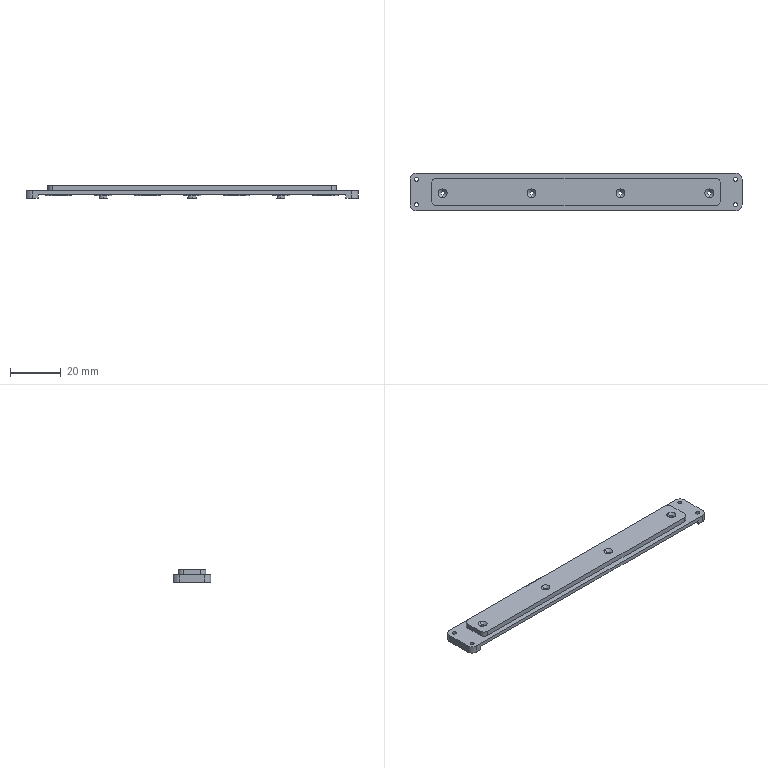NC program | NX | posted with a generic post | part box 130.666 x 14.95 x 5 mm
Lines 1701 to 3662 of 3855, first 1713 of 1960 lines:
(CAVITY_MILL_COPY_COPY , TOOL : D2)
N3370 T02 M6
N3372 G54
N3374 G17 G0 G90 X50.631 Y-0.725 S9500 M3
N3376 G43 Z30. H2
N3378 Z-0.125
N3380 G94 G1 Z-1.125 F1000.
N3382 X50.588 Y-0.761
N3384 G3 X50.231 Y-1.527 R1.
N3386 G1 Y-2.675 F1100.
N3388 X51.379
N3390 G3 X52.145 Y-2.318 R1.
N3392 G1 X52.181 Y-2.275
N3394 Z-0.125
N3396 G0 X50.631 Y-0.725 Z-0.25
N3398 G1 Z-1.25 F1000.
N3400 X50.588 Y-0.761
N3402 G3 X50.231 Y-1.527 R1.
N3404 G1 Y-2.675 F1100.
N3406 X51.379
N3408 G3 X52.145 Y-2.318 R1.
N3410 G1 X52.181 Y-2.275
N3412 Z-0.25
N3414 G0 X50.631 Y-0.725 Z-0.375
N3416 G1 Z-1.375 F1000.
N3418 X50.588 Y-0.761
N3420 G3 X50.231 Y-1.527 R1.
N3422 G1 Y-2.675 F1100.
N3424 X51.379
N3426 G3 X52.145 Y-2.318 R1.
N3428 G1 X52.181 Y-2.275
N3430 Z-0.375
N3432 G0 X50.631 Y-0.725 Z-0.5
N3434 G1 Z-1.5 F1000.
N3436 X50.588 Y-0.761
N3438 G3 X50.231 Y-1.527 R1.
N3440 G1 Y-2.675 F1100.
N3442 X51.379
N3444 G3 X52.145 Y-2.318 R1.
N3446 G1 X52.181 Y-2.275
N3448 Z-0.5
N3450 G0 X50.631 Y-0.725 Z-0.65
N3452 G1 Z-1.65 F1000.
N3454 X50.588 Y-0.761
N3456 G3 X50.231 Y-1.527 R1.
N3458 G1 Y-2.675 F1100.
N3460 X51.379
N3462 G3 X52.145 Y-2.318 R1.
N3464 G1 X52.181 Y-2.275
N3466 Z-0.65
N3468 G0 X50.631 Y-0.725 Z-0.8
N3470 G1 Z-1.8 F1000.
N3472 X50.588 Y-0.761
N3474 G3 X50.231 Y-1.527 R1.
N3476 G1 Y-2.675 F1100.
N3478 X51.379
N3480 G3 X52.145 Y-2.318 R1.
N3482 G1 X52.181 Y-2.275
N3484 Z-0.8
N3486 G0 X50.631 Y-0.725 Z-0.95
N3488 G1 Z-1.95 F1000.
N3490 X50.588 Y-0.761
N3492 G3 X50.231 Y-1.527 R1.
N3494 G1 Y-2.675 F1100.
N3496 X51.379
N3498 G3 X52.145 Y-2.318 R1.
N3500 G1 X52.181 Y-2.275
N3502 Z-0.95
N3504 G0 X50.631 Y-0.725 Z-1.1
N3506 G1 Z-2.1 F1000.
N3508 X50.588 Y-0.761
N3510 G3 X50.231 Y-1.527 R1.
N3512 G1 Y-2.675 F1100.
N3514 X51.379
N3516 G3 X52.145 Y-2.318 R1.
N3518 G1 X52.181 Y-2.275
N3520 Z-1.1
N3522 G0 X50.631 Y-0.725 Z-1.25
N3524 G1 Z-2.25 F1000.
N3526 X50.588 Y-0.761
N3528 G3 X50.231 Y-1.527 R1.
N3530 G1 Y-2.675 F1100.
N3532 X51.379
N3534 G3 X52.145 Y-2.318 R1.
N3536 G1 X52.181 Y-2.275
N3538 Z-1.25
N3540 G0 X50.631 Y-0.725 Z-1.4
N3542 G1 Z-2.4 F1000.
N3544 X50.588 Y-0.761
N3546 G3 X50.231 Y-1.527 R1.
N3548 G1 Y-2.675 F1100.
N3550 X51.379
N3552 G3 X52.145 Y-2.318 R1.
N3554 G1 X52.181 Y-2.275
N3556 Z-1.4
N3558 G0 X50.631 Y-0.725 Z-1.55
N3560 G1 Z-2.55 F1000.
N3562 X50.588 Y-0.761
N3564 G3 X50.231 Y-1.527 R1.
N3566 G1 Y-2.675 F1100.
N3568 X51.379
N3570 G3 X52.145 Y-2.318 R1.
N3572 G1 X52.181 Y-2.275
N3574 Z-1.55
N3576 G0 X50.631 Y-0.725 Z-1.7
N3578 G1 Z-2.7 F1000.
N3580 X50.588 Y-0.761
N3582 G3 X50.231 Y-1.527 R1.
N3584 G1 Y-2.675 F1100.
N3586 X51.379
N3588 G3 X52.145 Y-2.318 R1.
N3590 G1 X52.181 Y-2.275
N3592 Z-1.7
N3594 G0 Z30.
N3596 X52.83
N3598 Z-0.125
N3600 G1 Z-1.125 F1000.
N3602 X52.866 Y-2.318
N3604 G3 X53.632 Y-2.675 R1.
N3606 G1 X54.781 F1100.
N3608 Y-1.527
N3610 G3 X54.424 Y-0.761 R1.
N3612 G1 X54.381 Y-0.725
N3614 Z-0.125
N3616 G0 X52.83 Y-2.275 Z-0.25
N3618 G1 Z-1.25 F1000.
N3620 X52.866 Y-2.318
N3622 G3 X53.632 Y-2.675 R1.
N3624 G1 X54.781 F1100.
N3626 Y-1.527
N3628 G3 X54.424 Y-0.761 R1.
N3630 G1 X54.381 Y-0.725
N3632 Z-0.25
N3634 G0 X52.83 Y-2.275 Z-0.375
N3636 G1 Z-1.375 F1000.
N3638 X52.866 Y-2.318
N3640 G3 X53.632 Y-2.675 R1.
N3642 G1 X54.781 F1100.
N3644 Y-1.527
N3646 G3 X54.424 Y-0.761 R1.
N3648 G1 X54.381 Y-0.725
N3650 Z-0.375
N3652 G0 X52.83 Y-2.275 Z-0.5
N3654 G1 Z-1.5 F1000.
N3656 X52.866 Y-2.318
N3658 G3 X53.632 Y-2.675 R1.
N3660 G1 X54.781 F1100.
N3662 Y-1.527
N3664 G3 X54.424 Y-0.761 R1.
N3666 G1 X54.381 Y-0.725
N3668 Z-0.5
N3670 G0 X52.83 Y-2.275 Z-0.65
N3672 G1 Z-1.65 F1000.
N3674 X52.866 Y-2.318
N3676 G3 X53.632 Y-2.675 R1.
N3678 G1 X54.781 F1100.
N3680 Y-1.527
N3682 G3 X54.424 Y-0.761 R1.
N3684 G1 X54.381 Y-0.725
N3686 Z-0.65
N3688 G0 X52.83 Y-2.275 Z-0.8
N3690 G1 Z-1.8 F1000.
N3692 X52.866 Y-2.318
N3694 G3 X53.632 Y-2.675 R1.
N3696 G1 X54.781 F1100.
N3698 Y-1.527
N3700 G3 X54.424 Y-0.761 R1.
N3702 G1 X54.381 Y-0.725
N3704 Z-0.8
N3706 G0 X52.83 Y-2.275 Z-0.95
N3708 G1 Z-1.95 F1000.
N3710 X52.866 Y-2.318
N3712 G3 X53.632 Y-2.675 R1.
N3714 G1 X54.781 F1100.
N3716 Y-1.527
N3718 G3 X54.424 Y-0.761 R1.
N3720 G1 X54.381 Y-0.725
N3722 Z-0.95
N3724 G0 X52.83 Y-2.275 Z-1.1
N3726 G1 Z-2.1 F1000.
N3728 X52.866 Y-2.318
N3730 G3 X53.632 Y-2.675 R1.
N3732 G1 X54.781 F1100.
N3734 Y-1.527
N3736 G3 X54.424 Y-0.761 R1.
N3738 G1 X54.381 Y-0.725
N3740 Z-1.1
N3742 G0 X52.83 Y-2.275 Z-1.25
N3744 G1 Z-2.25 F1000.
N3746 X52.866 Y-2.318
N3748 G3 X53.632 Y-2.675 R1.
N3750 G1 X54.781 F1100.
N3752 Y-1.527
N3754 G3 X54.424 Y-0.761 R1.
N3756 G1 X54.381 Y-0.725
N3758 Z-1.25
N3760 G0 X52.83 Y-2.275 Z-1.4
N3762 G1 Z-2.4 F1000.
N3764 X52.866 Y-2.318
N3766 G3 X53.632 Y-2.675 R1.
N3768 G1 X54.781 F1100.
N3770 Y-1.527
N3772 G3 X54.424 Y-0.761 R1.
N3774 G1 X54.381 Y-0.725
N3776 Z-1.4
N3778 G0 X52.83 Y-2.275 Z-1.55
N3780 G1 Z-2.55 F1000.
N3782 X52.866 Y-2.318
N3784 G3 X53.632 Y-2.675 R1.
N3786 G1 X54.781 F1100.
N3788 Y-1.527
N3790 G3 X54.424 Y-0.761 R1.
N3792 G1 X54.381 Y-0.725
N3794 Z-1.55
N3796 G0 X52.83 Y-2.275 Z-1.7
N3798 G1 Z-2.7 F1000.
N3800 X52.866 Y-2.318
N3802 G3 X53.632 Y-2.675 R1.
N3804 G1 X54.781 F1100.
N3806 Y-1.527
N3808 G3 X54.424 Y-0.761 R1.
N3810 G1 X54.381 Y-0.725
N3812 Z-1.7
N3814 G0 Z30.
N3816 X57.814 Y-5.892
N3818 Z-0.125
N3820 G1 Z-1.125 F1000.
N3822 G2 X58.204 Y-5.422 R1.
N3824 X59.034 Y-5.708 R0.56 F1100.
N3826 G3 X59.506 Y-6.042 R0.5
N3828 G1 Y6.042
N3830 G3 X59.034 Y5.708 R0.5
N3832 G2 X58.204 Y5.422 R0.56
N3834 G3 X57.617 Y5.387 R0.5
N3836 G2 X58.581 Y2.975 R3.5
N3838 G1 Y-2.975
N3840 G2 X57.617 Y-5.387 R3.5
N3842 G3 X58.204 Y-5.422 R0.5
N3844 G2 X59.042 Y-5.31 R1.
N3846 G1 X58.614 Y-5.776
N3848 Z-0.125
N3850 G0 X57.814 Y-5.892 Z-0.25
N3852 G1 Z-1.25 F1000.
N3854 G2 X58.204 Y-5.422 R1.
N3856 X59.034 Y-5.708 R0.56 F1100.
N3858 G3 X59.506 Y-6.042 R0.5
N3860 G1 Y6.042
N3862 G3 X59.034 Y5.708 R0.5
N3864 G2 X58.204 Y5.422 R0.56
N3866 G3 X57.617 Y5.387 R0.5
N3868 G2 X58.581 Y2.975 R3.5
N3870 G1 Y-2.975
N3872 G2 X57.617 Y-5.387 R3.5
N3874 G3 X58.204 Y-5.422 R0.5
N3876 G2 X59.042 Y-5.31 R1.
N3878 G1 X58.614 Y-5.776
N3880 Z-0.25
N3882 G0 X57.814 Y-5.892 Z-0.375
N3884 G1 Z-1.375 F1000.
N3886 G2 X58.204 Y-5.422 R1.
N3888 X59.034 Y-5.708 R0.56 F1100.
N3890 G3 X59.506 Y-6.042 R0.5
N3892 G1 Y6.042
N3894 G3 X59.034 Y5.708 R0.5
N3896 G2 X58.204 Y5.422 R0.56
N3898 G3 X57.617 Y5.387 R0.5
N3900 G2 X58.581 Y2.975 R3.5
N3902 G1 Y-2.975
N3904 G2 X57.617 Y-5.387 R3.5
N3906 G3 X58.204 Y-5.422 R0.5
N3908 G2 X59.042 Y-5.31 R1.
N3910 G1 X58.614 Y-5.776
N3912 Z-0.375
N3914 G0 X57.814 Y-5.892 Z-0.5
N3916 G1 Z-1.5 F1000.
N3918 G2 X58.204 Y-5.422 R1.
N3920 X59.034 Y-5.708 R0.56 F1100.
N3922 G3 X59.506 Y-6.042 R0.5
N3924 G1 Y6.042
N3926 G3 X59.034 Y5.708 R0.5
N3928 G2 X58.204 Y5.422 R0.56
N3930 G3 X57.617 Y5.387 R0.5
N3932 G2 X58.581 Y2.975 R3.5
N3934 G1 Y-2.975
N3936 G2 X57.617 Y-5.387 R3.5
N3938 G3 X58.204 Y-5.422 R0.5
N3940 G2 X59.042 Y-5.31 R1.
N3942 G1 X58.614 Y-5.776
N3944 Z-0.5
N3946 G0 Z30.
N3948 X54.381 Y0.725
N3950 Z-0.125
N3952 G1 Z-1.125 F1000.
N3954 X54.424 Y0.761
N3956 G3 X54.781 Y1.527 R1.
N3958 G1 Y2.595 F1100.
N3960 X54.779 Y2.675
N3962 X54.588
N3964 X53.632
N3966 G3 X52.866 Y2.318 R1.
N3968 G1 X52.83 Y2.275
N3970 Z-0.125
N3972 G0 X54.381 Y0.725 Z-0.25
N3974 G1 Z-1.25 F1000.
N3976 X54.424 Y0.761
N3978 G3 X54.781 Y1.527 R1.
N3980 G1 Y2.595 F1100.
N3982 X54.779 Y2.675
N3984 X54.588
N3986 X53.632
N3988 G3 X52.866 Y2.318 R1.
N3990 G1 X52.83 Y2.275
N3992 Z-0.25
N3994 G0 X54.381 Y0.725 Z-0.375
N3996 G1 Z-1.375 F1000.
N3998 X54.424 Y0.761
N4000 G3 X54.781 Y1.527 R1.
N4002 G1 Y2.595 F1100.
N4004 X54.779 Y2.675
N4006 X53.632
N4008 G3 X52.866 Y2.318 R1.
N4010 G1 X52.83 Y2.275
N4012 Z-0.375
N4014 G0 X54.381 Y0.725 Z-0.5
N4016 G1 Z-1.5 F1000.
N4018 X54.424 Y0.761
N4020 G3 X54.781 Y1.527 R1.
N4022 G1 Y2.595 F1100.
N4024 X54.779 Y2.675
N4026 X53.632
N4028 G3 X52.866 Y2.318 R1.
N4030 G1 X52.83 Y2.275
N4032 Z-0.5
N4034 G0 X54.381 Y0.725 Z-0.65
N4036 G1 Z-1.65 F1000.
N4038 X54.424 Y0.761
N4040 G3 X54.781 Y1.527 R1.
N4042 G1 Y2.595 F1100.
N4044 X54.779 Y2.675
N4046 X53.632
N4048 G3 X52.866 Y2.318 R1.
N4050 G1 X52.83 Y2.275
N4052 Z-0.65
N4054 G0 X54.381 Y0.725 Z-0.8
N4056 G1 Z-1.8 F1000.
N4058 X54.424 Y0.761
N4060 G3 X54.781 Y1.527 R1.
N4062 G1 Y2.595 F1100.
N4064 X54.779 Y2.675
N4066 X53.632
N4068 G3 X52.866 Y2.318 R1.
N4070 G1 X52.83 Y2.275
N4072 Z-0.8
N4074 G0 X54.381 Y0.725 Z-0.95
N4076 G1 Z-1.95 F1000.
N4078 X54.424 Y0.761
N4080 G3 X54.781 Y1.527 R1.
N4082 G1 Y2.595 F1100.
N4084 X54.779 Y2.675
N4086 X53.632
N4088 G3 X52.866 Y2.318 R1.
N4090 G1 X52.83 Y2.275
N4092 Z-0.95
N4094 G0 X54.381 Y0.725 Z-1.1
N4096 G1 Z-2.1 F1000.
N4098 X54.424 Y0.761
N4100 G3 X54.781 Y1.527 R1.
N4102 G1 Y2.595 F1100.
N4104 X54.779 Y2.675
N4106 X53.632
N4108 G3 X52.866 Y2.318 R1.
N4110 G1 X52.83 Y2.275
N4112 Z-1.1
N4114 G0 X54.381 Y0.725 Z-1.25
N4116 G1 Z-2.25 F1000.
N4118 X54.424 Y0.761
N4120 G3 X54.781 Y1.527 R1.
N4122 G1 Y2.595 F1100.
N4124 X54.779 Y2.675
N4126 X53.632
N4128 G3 X52.866 Y2.318 R1.
N4130 G1 X52.83 Y2.275
N4132 Z-1.25
N4134 G0 X54.381 Y0.725 Z-1.4
N4136 G1 Z-2.4 F1000.
N4138 X54.424 Y0.761
N4140 G3 X54.781 Y1.527 R1.
N4142 G1 Y2.595 F1100.
N4144 X54.778 Y2.675
N4146 X53.632
N4148 G3 X52.866 Y2.318 R1.
N4150 G1 X52.83 Y2.275
N4152 Z-1.4
N4154 G0 X54.381 Y0.725 Z-1.55
N4156 G1 Z-2.55 F1000.
N4158 X54.424 Y0.761
N4160 G3 X54.781 Y1.527 R1.
N4162 G1 Y2.595 F1100.
N4164 X54.778 Y2.675
N4166 X53.632
N4168 G3 X52.866 Y2.318 R1.
N4170 G1 X52.83 Y2.275
N4172 Z-1.55
N4174 G0 X54.381 Y0.725 Z-1.7
N4176 G1 Z-2.7 F1000.
N4178 X54.424 Y0.761
N4180 G3 X54.781 Y1.527 R1.
N4182 G1 Y2.595 F1100.
N4184 X54.778 Y2.675
N4186 X53.632
N4188 G3 X52.866 Y2.318 R1.
N4190 G1 X52.83 Y2.275
N4192 Z-1.7
N4194 G0 Z30.
N4196 X52.181
N4198 Z-0.125
N4200 G1 Z-1.125 F1000.
N4202 X52.145 Y2.318
N4204 G3 X51.379 Y2.675 R1.
N4206 G1 X50.231 F1100.
N4208 Y1.527
N4210 G3 X50.588 Y0.761 R1.
N4212 G1 X50.631 Y0.725
N4214 Z-0.125
N4216 G0 X52.181 Y2.275 Z-0.25
N4218 G1 Z-1.25 F1000.
N4220 X52.145 Y2.318
N4222 G3 X51.379 Y2.675 R1.
N4224 G1 X50.231 F1100.
N4226 Y1.527
N4228 G3 X50.588 Y0.761 R1.
N4230 G1 X50.631 Y0.725
N4232 Z-0.25
N4234 G0 X52.181 Y2.275 Z-0.375
N4236 G1 Z-1.375 F1000.
N4238 X52.145 Y2.318
N4240 G3 X51.379 Y2.675 R1.
N4242 G1 X50.231 F1100.
N4244 Y1.527
N4246 G3 X50.588 Y0.761 R1.
N4248 G1 X50.631 Y0.725
N4250 Z-0.375
N4252 G0 X52.181 Y2.275 Z-0.5
N4254 G1 Z-1.5 F1000.
N4256 X52.145 Y2.318
N4258 G3 X51.379 Y2.675 R1.
N4260 G1 X50.231 F1100.
N4262 Y1.527
N4264 G3 X50.588 Y0.761 R1.
N4266 G1 X50.631 Y0.725
N4268 Z-0.5
N4270 G0 X52.181 Y2.275 Z-0.65
N4272 G1 Z-1.65 F1000.
N4274 X52.145 Y2.318
N4276 G3 X51.379 Y2.675 R1.
N4278 G1 X50.231 F1100.
N4280 Y1.527
N4282 G3 X50.588 Y0.761 R1.
N4284 G1 X50.631 Y0.725
N4286 Z-0.65
N4288 G0 X52.181 Y2.275 Z-0.8
N4290 G1 Z-1.8 F1000.
N4292 X52.145 Y2.318
N4294 G3 X51.379 Y2.675 R1.
N4296 G1 X50.231 F1100.
N4298 Y1.527
N4300 G3 X50.588 Y0.761 R1.
N4302 G1 X50.631 Y0.725
N4304 Z-0.8
N4306 G0 X52.181 Y2.275 Z-0.95
N4308 G1 Z-1.95 F1000.
N4310 X52.145 Y2.318
N4312 G3 X51.379 Y2.675 R1.
N4314 G1 X50.231 F1100.
N4316 Y1.527
N4318 G3 X50.588 Y0.761 R1.
N4320 G1 X50.631 Y0.725
N4322 Z-0.95
N4324 G0 X52.181 Y2.275 Z-1.1
N4326 G1 Z-2.1 F1000.
N4328 X52.145 Y2.318
N4330 G3 X51.379 Y2.675 R1.
N4332 G1 X50.231 F1100.
N4334 Y1.527
N4336 G3 X50.588 Y0.761 R1.
N4338 G1 X50.631 Y0.725
N4340 Z-1.1
N4342 G0 X52.181 Y2.275 Z-1.25
N4344 G1 Z-2.25 F1000.
N4346 X52.145 Y2.318
N4348 G3 X51.379 Y2.675 R1.
N4350 G1 X50.231 F1100.
N4352 Y1.527
N4354 G3 X50.588 Y0.761 R1.
N4356 G1 X50.631 Y0.725
N4358 Z-1.25
N4360 G0 X52.181 Y2.275 Z-1.4
N4362 G1 Z-2.4 F1000.
N4364 X52.145 Y2.318
N4366 G3 X51.379 Y2.675 R1.
N4368 G1 X50.231 F1100.
N4370 Y1.527
N4372 G3 X50.588 Y0.761 R1.
N4374 G1 X50.631 Y0.725
N4376 Z-1.4
N4378 G0 X52.181 Y2.275 Z-1.55
N4380 G1 Z-2.55 F1000.
N4382 X52.145 Y2.318
N4384 G3 X51.379 Y2.675 R1.
N4386 G1 X50.231 F1100.
N4388 Y1.527
N4390 G3 X50.588 Y0.761 R1.
N4392 G1 X50.631 Y0.725
N4394 Z-1.55
N4396 G0 X52.181 Y2.275 Z-1.7
N4398 G1 Z-2.7 F1000.
N4400 X52.145 Y2.318
N4402 G3 X51.379 Y2.675 R1.
N4404 G1 X50.231 F1100.
N4406 Y1.527
N4408 G3 X50.588 Y0.761 R1.
N4410 G1 X50.631 Y0.725
N4412 Z-1.7
N4414 G0 Z30.
N4416 X19.381
N4418 Z-0.125
N4420 G1 Z-1.125 F1000.
N4422 X19.424 Y0.761
N4424 G3 X19.781 Y1.527 R1.
N4426 G1 Y2.675 F1100.
N4428 X18.632
N4430 G3 X17.866 Y2.318 R1.
N4432 G1 X17.83 Y2.275
N4434 Z-0.125
N4436 G0 X19.381 Y0.725 Z-0.25
N4438 G1 Z-1.25 F1000.
N4440 X19.424 Y0.761
N4442 G3 X19.781 Y1.527 R1.
N4444 G1 Y2.675 F1100.
N4446 X18.632
N4448 G3 X17.866 Y2.318 R1.
N4450 G1 X17.83 Y2.275
N4452 Z-0.25
N4454 G0 X19.381 Y0.725 Z-0.375
N4456 G1 Z-1.375 F1000.
N4458 X19.424 Y0.761
N4460 G3 X19.781 Y1.527 R1.
N4462 G1 Y2.675 F1100.
N4464 X18.632
N4466 G3 X17.866 Y2.318 R1.
N4468 G1 X17.83 Y2.275
N4470 Z-0.375
N4472 G0 X19.381 Y0.725 Z-0.5
N4474 G1 Z-1.5 F1000.
N4476 X19.424 Y0.761
N4478 G3 X19.781 Y1.527 R1.
N4480 G1 Y2.675 F1100.
N4482 X18.632
N4484 G3 X17.866 Y2.318 R1.
N4486 G1 X17.83 Y2.275
N4488 Z-0.5
N4490 G0 X19.381 Y0.725 Z-0.65
N4492 G1 Z-1.65 F1000.
N4494 X19.424 Y0.761
N4496 G3 X19.781 Y1.527 R1.
N4498 G1 Y2.675 F1100.
N4500 X18.632
N4502 G3 X17.866 Y2.318 R1.
N4504 G1 X17.83 Y2.275
N4506 Z-0.65
N4508 G0 X19.381 Y0.725 Z-0.8
N4510 G1 Z-1.8 F1000.
N4512 X19.424 Y0.761
N4514 G3 X19.781 Y1.527 R1.
N4516 G1 Y2.675 F1100.
N4518 X18.632
N4520 G3 X17.866 Y2.318 R1.
N4522 G1 X17.83 Y2.275
N4524 Z-0.8
N4526 G0 X19.381 Y0.725 Z-0.95
N4528 G1 Z-1.95 F1000.
N4530 X19.424 Y0.761
N4532 G3 X19.781 Y1.527 R1.
N4534 G1 Y2.675 F1100.
N4536 X18.632
N4538 G3 X17.866 Y2.318 R1.
N4540 G1 X17.83 Y2.275
N4542 Z-0.95
N4544 G0 X19.381 Y0.725 Z-1.1
N4546 G1 Z-2.1 F1000.
N4548 X19.424 Y0.761
N4550 G3 X19.781 Y1.527 R1.
N4552 G1 Y2.675 F1100.
N4554 X18.632
N4556 G3 X17.866 Y2.318 R1.
N4558 G1 X17.83 Y2.275
N4560 Z-1.1
N4562 G0 X19.381 Y0.725 Z-1.25
N4564 G1 Z-2.25 F1000.
N4566 X19.424 Y0.761
N4568 G3 X19.781 Y1.527 R1.
N4570 G1 Y2.675 F1100.
N4572 X18.632
N4574 G3 X17.866 Y2.318 R1.
N4576 G1 X17.83 Y2.275
N4578 Z-1.25
N4580 G0 X19.381 Y0.725 Z-1.4
N4582 G1 Z-2.4 F1000.
N4584 X19.424 Y0.761
N4586 G3 X19.781 Y1.527 R1.
N4588 G1 Y2.675 F1100.
N4590 X18.632
N4592 G3 X17.866 Y2.318 R1.
N4594 G1 X17.83 Y2.275
N4596 Z-1.4
N4598 G0 X19.381 Y0.725 Z-1.55
N4600 G1 Z-2.55 F1000.
N4602 X19.424 Y0.761
N4604 G3 X19.781 Y1.527 R1.
N4606 G1 Y2.675 F1100.
N4608 X18.632
N4610 G3 X17.866 Y2.318 R1.
N4612 G1 X17.83 Y2.275
N4614 Z-1.55
N4616 G0 X19.381 Y0.725 Z-1.7
N4618 G1 Z-2.7 F1000.
N4620 X19.424 Y0.761
N4622 G3 X19.781 Y1.527 R1.
N4624 G1 Y2.675 F1100.
N4626 X18.632
N4628 G3 X17.866 Y2.318 R1.
N4630 G1 X17.83 Y2.275
N4632 Z-1.7
N4634 G0 Z30.
N4636 Y-2.275
N4638 Z-0.125
N4640 G1 Z-1.125 F1000.
N4642 X17.866 Y-2.318
N4644 G3 X18.632 Y-2.675 R1.
N4646 G1 X19.781 F1100.
N4648 Y-1.527
N4650 G3 X19.424 Y-0.761 R1.
N4652 G1 X19.381 Y-0.725
N4654 Z-0.125
N4656 G0 X17.83 Y-2.275 Z-0.25
N4658 G1 Z-1.25 F1000.
N4660 X17.866 Y-2.318
N4662 G3 X18.632 Y-2.675 R1.
N4664 G1 X19.781 F1100.
N4666 Y-1.527
N4668 G3 X19.424 Y-0.761 R1.
N4670 G1 X19.381 Y-0.725
N4672 Z-0.25
N4674 G0 X17.83 Y-2.275 Z-0.375
N4676 G1 Z-1.375 F1000.
N4678 X17.866 Y-2.318
N4680 G3 X18.632 Y-2.675 R1.
N4682 G1 X19.781 F1100.
N4684 Y-1.527
N4686 G3 X19.424 Y-0.761 R1.
N4688 G1 X19.381 Y-0.725
N4690 Z-0.375
N4692 G0 X17.83 Y-2.275 Z-0.5
N4694 G1 Z-1.5 F1000.
N4696 X17.866 Y-2.318
N4698 G3 X18.632 Y-2.675 R1.
N4700 G1 X19.781 F1100.
N4702 Y-1.527
N4704 G3 X19.424 Y-0.761 R1.
N4706 G1 X19.381 Y-0.725
N4708 Z-0.5
N4710 G0 X17.83 Y-2.275 Z-0.65
N4712 G1 Z-1.65 F1000.
N4714 X17.866 Y-2.318
N4716 G3 X18.632 Y-2.675 R1.
N4718 G1 X19.781 F1100.
N4720 Y-1.527
N4722 G3 X19.424 Y-0.761 R1.
N4724 G1 X19.381 Y-0.725
N4726 Z-0.65
N4728 G0 X17.83 Y-2.275 Z-0.8
N4730 G1 Z-1.8 F1000.
N4732 X17.866 Y-2.318
N4734 G3 X18.632 Y-2.675 R1.
N4736 G1 X19.781 F1100.
N4738 Y-1.527
N4740 G3 X19.424 Y-0.761 R1.
N4742 G1 X19.381 Y-0.725
N4744 Z-0.8
N4746 G0 X17.83 Y-2.275 Z-0.95
N4748 G1 Z-1.95 F1000.
N4750 X17.866 Y-2.318
N4752 G3 X18.632 Y-2.675 R1.
N4754 G1 X19.781 F1100.
N4756 Y-1.527
N4758 G3 X19.424 Y-0.761 R1.
N4760 G1 X19.381 Y-0.725
N4762 Z-0.95
N4764 G0 X17.83 Y-2.275 Z-1.1
N4766 G1 Z-2.1 F1000.
N4768 X17.866 Y-2.318
N4770 G3 X18.632 Y-2.675 R1.
N4772 G1 X19.781 F1100.
N4774 Y-1.527
N4776 G3 X19.424 Y-0.761 R1.
N4778 G1 X19.381 Y-0.725
N4780 Z-1.1
N4782 G0 X17.83 Y-2.275 Z-1.25
N4784 G1 Z-2.25 F1000.
N4786 X17.866 Y-2.318
N4788 G3 X18.632 Y-2.675 R1.
N4790 G1 X19.781 F1100.
N4792 Y-1.527
N4794 G3 X19.424 Y-0.761 R1.
N4796 G1 X19.381 Y-0.725
N4798 Z-1.25
N4800 G0 X17.83 Y-2.275 Z-1.4
N4802 G1 Z-2.4 F1000.
N4804 X17.866 Y-2.318
N4806 G3 X18.632 Y-2.675 R1.
N4808 G1 X19.781 F1100.
N4810 Y-1.527
N4812 G3 X19.424 Y-0.761 R1.
N4814 G1 X19.381 Y-0.725
N4816 Z-1.4
N4818 G0 X17.83 Y-2.275 Z-1.55
N4820 G1 Z-2.55 F1000.
N4822 X17.866 Y-2.318
N4824 G3 X18.632 Y-2.675 R1.
N4826 G1 X19.781 F1100.
N4828 Y-1.527
N4830 G3 X19.424 Y-0.761 R1.
N4832 G1 X19.381 Y-0.725
N4834 Z-1.55
N4836 G0 X17.83 Y-2.275 Z-1.7
N4838 G1 Z-2.7 F1000.
N4840 X17.866 Y-2.318
N4842 G3 X18.632 Y-2.675 R1.
N4844 G1 X19.781 F1100.
N4846 Y-1.527
N4848 G3 X19.424 Y-0.761 R1.
N4850 G1 X19.381 Y-0.725
N4852 Z-1.7
N4854 G0 Z30.
N4856 X15.631
N4858 Z-0.125
N4860 G1 Z-1.125 F1000.
N4862 X15.588 Y-0.761
N4864 G3 X15.231 Y-1.527 R1.
N4866 G1 Y-2.675 F1100.
N4868 X16.379
N4870 G3 X17.145 Y-2.318 R1.
N4872 G1 X17.181 Y-2.275
N4874 Z-0.125
N4876 G0 X15.631 Y-0.725 Z-0.25
N4878 G1 Z-1.25 F1000.
N4880 X15.588 Y-0.761
N4882 G3 X15.231 Y-1.527 R1.
N4884 G1 Y-2.675 F1100.
N4886 X16.379
N4888 G3 X17.145 Y-2.318 R1.
N4890 G1 X17.181 Y-2.275
N4892 Z-0.25
N4894 G0 X15.631 Y-0.725 Z-0.375
N4896 G1 Z-1.375 F1000.
N4898 X15.588 Y-0.761
N4900 G3 X15.231 Y-1.527 R1.
N4902 G1 Y-2.675 F1100.
N4904 X16.379
N4906 G3 X17.145 Y-2.318 R1.
N4908 G1 X17.181 Y-2.275
N4910 Z-0.375
N4912 G0 X15.631 Y-0.725 Z-0.5
N4914 G1 Z-1.5 F1000.
N4916 X15.588 Y-0.761
N4918 G3 X15.231 Y-1.527 R1.
N4920 G1 Y-2.675 F1100.
N4922 X16.379
N4924 G3 X17.145 Y-2.318 R1.
N4926 G1 X17.181 Y-2.275
N4928 Z-0.5
N4930 G0 X15.631 Y-0.725 Z-0.65
N4932 G1 Z-1.65 F1000.
N4934 X15.588 Y-0.761
N4936 G3 X15.231 Y-1.527 R1.
N4938 G1 Y-2.675 F1100.
N4940 X16.379
N4942 G3 X17.145 Y-2.318 R1.
N4944 G1 X17.181 Y-2.275
N4946 Z-0.65
N4948 G0 X15.631 Y-0.725 Z-0.8
N4950 G1 Z-1.8 F1000.
N4952 X15.588 Y-0.761
N4954 G3 X15.231 Y-1.527 R1.
N4956 G1 Y-2.675 F1100.
N4958 X16.379
N4960 G3 X17.145 Y-2.318 R1.
N4962 G1 X17.181 Y-2.275
N4964 Z-0.8
N4966 G0 X15.631 Y-0.725 Z-0.95
N4968 G1 Z-1.95 F1000.
N4970 X15.588 Y-0.761
N4972 G3 X15.231 Y-1.527 R1.
N4974 G1 Y-2.675 F1100.
N4976 X16.379
N4978 G3 X17.145 Y-2.318 R1.
N4980 G1 X17.181 Y-2.275
N4982 Z-0.95
N4984 G0 X15.631 Y-0.725 Z-1.1
N4986 G1 Z-2.1 F1000.
N4988 X15.588 Y-0.761
N4990 G3 X15.231 Y-1.527 R1.
N4992 G1 Y-2.675 F1100.
N4994 X16.379
N4996 G3 X17.145 Y-2.318 R1.
N4998 G1 X17.181 Y-2.275
N5000 Z-1.1
N5002 G0 X15.631 Y-0.725 Z-1.25
N5004 G1 Z-2.25 F1000.
N5006 X15.588 Y-0.761
N5008 G3 X15.231 Y-1.527 R1.
N5010 G1 X15.232 Y-2.675 F1100.
N5012 X16.379
N5014 G3 X17.145 Y-2.318 R1.
N5016 G1 X17.181 Y-2.275
N5018 Z-1.25
N5020 G0 X15.631 Y-0.725 Z-1.4
N5022 G1 Z-2.4 F1000.
N5024 X15.588 Y-0.761
N5026 G3 X15.231 Y-1.527 R1.
N5028 G1 X15.232 Y-2.675 F1100.
N5030 X16.379
N5032 G3 X17.145 Y-2.318 R1.
N5034 G1 X17.181 Y-2.275
N5036 Z-1.4
N5038 G0 X15.631 Y-0.725 Z-1.55
N5040 G1 Z-2.55 F1000.
N5042 X15.588 Y-0.761
N5044 G3 X15.231 Y-1.527 R1.
N5046 G1 X15.232 Y-2.675 F1100.
N5048 X16.379
N5050 G3 X17.145 Y-2.318 R1.
N5052 G1 X17.181 Y-2.275
N5054 Z-1.55
N5056 G0 X15.631 Y-0.725 Z-1.7
N5058 G1 Z-2.7 F1000.
N5060 X15.588 Y-0.761
N5062 G3 X15.231 Y-1.527 R1.
N5064 G1 X15.232 Y-2.675 F1100.
N5066 X16.379
N5068 G3 X17.145 Y-2.318 R1.
N5070 G1 X17.181 Y-2.275
N5072 Z-1.7
N5074 G0 Z30.
N5076 Y2.275
N5078 Z-0.125
N5080 G1 Z-1.125 F1000.
N5082 X17.145 Y2.318
N5084 G3 X16.379 Y2.675 R1.
N5086 G1 X15.547 F1100.
N5088 X15.231
N5090 Y1.527
N5092 G3 X15.588 Y0.761 R1.
N5094 G1 X15.631 Y0.725
N5096 Z-0.125
N5098 G0 X17.181 Y2.275 Z-0.25
N5100 G1 Z-1.25 F1000.
N5102 X17.145 Y2.318
N5104 G3 X16.379 Y2.675 R1.
N5106 G1 X15.547 F1100.
N5108 X15.231
N5110 Y1.527
N5112 G3 X15.588 Y0.761 R1.
N5114 G1 X15.631 Y0.725
N5116 Z-0.25
N5118 G0 X17.181 Y2.275 Z-0.375
N5120 G1 Z-1.375 F1000.
N5122 X17.145 Y2.318
N5124 G3 X16.379 Y2.675 R1.
N5126 G1 X15.547 F1100.
N5128 X15.231
N5130 Y1.527
N5132 G3 X15.588 Y0.761 R1.
N5134 G1 X15.631 Y0.725
N5136 Z-0.375
N5138 G0 X17.181 Y2.275 Z-0.5
N5140 G1 Z-1.5 F1000.
N5142 X17.145 Y2.318
N5144 G3 X16.379 Y2.675 R1.
N5146 G1 X15.547 F1100.
N5148 X15.231
N5150 Y1.527
N5152 G3 X15.588 Y0.761 R1.
N5154 G1 X15.631 Y0.725
N5156 Z-0.5
N5158 G0 X17.181 Y2.275 Z-0.65
N5160 G1 Z-1.65 F1000.
N5162 X17.145 Y2.318
N5164 G3 X16.379 Y2.675 R1.
N5166 G1 X15.547 F1100.
N5168 X15.231
N5170 Y1.527
N5172 G3 X15.588 Y0.761 R1.
N5174 G1 X15.631 Y0.725
N5176 Z-0.65
N5178 G0 X17.181 Y2.275 Z-0.8
N5180 G1 Z-1.8 F1000.
N5182 X17.145 Y2.318
N5184 G3 X16.379 Y2.675 R1.
N5186 G1 X15.547 F1100.
N5188 X15.231
N5190 Y1.527
N5192 G3 X15.588 Y0.761 R1.
N5194 G1 X15.631 Y0.725
N5196 Z-0.8
N5198 G0 X17.181 Y2.275 Z-0.95
N5200 G1 Z-1.95 F1000.
N5202 X17.145 Y2.318
N5204 G3 X16.379 Y2.675 R1.
N5206 G1 X15.547 F1100.
N5208 X15.231
N5210 Y1.527
N5212 G3 X15.588 Y0.761 R1.
N5214 G1 X15.631 Y0.725
N5216 Z-0.95
N5218 G0 X17.181 Y2.275 Z-1.1
N5220 G1 Z-2.1 F1000.
N5222 X17.145 Y2.318
N5224 G3 X16.379 Y2.675 R1.
N5226 G1 X15.231 F1100.
N5228 Y1.527
N5230 G3 X15.588 Y0.761 R1.
N5232 G1 X15.631 Y0.725
N5234 Z-1.1
N5236 G0 X17.181 Y2.275 Z-1.25
N5238 G1 Z-2.25 F1000.
N5240 X17.145 Y2.318
N5242 G3 X16.379 Y2.675 R1.
N5244 G1 X15.231 Y2.674 F1100.
N5246 Y1.527
N5248 G3 X15.588 Y0.761 R1.
N5250 G1 X15.631 Y0.725
N5252 Z-1.25
N5254 G0 X17.181 Y2.275 Z-1.4
N5256 G1 Z-2.4 F1000.
N5258 X17.145 Y2.318
N5260 G3 X16.379 Y2.675 R1.
N5262 G1 X15.231 Y2.674 F1100.
N5264 Y1.527
N5266 G3 X15.588 Y0.761 R1.
N5268 G1 X15.631 Y0.725
N5270 Z-1.4
N5272 G0 X17.181 Y2.275 Z-1.55
N5274 G1 Z-2.55 F1000.
N5276 X17.145 Y2.318
N5278 G3 X16.379 Y2.675 R1.
N5280 G1 X15.231 Y2.674 F1100.
N5282 Y1.527
N5284 G3 X15.588 Y0.761 R1.
N5286 G1 X15.631 Y0.725
N5288 Z-1.55
N5290 G0 X17.181 Y2.275 Z-1.7
N5292 G1 Z-2.7 F1000.
N5294 X17.145 Y2.318
N5296 G3 X16.379 Y2.675 R1.
N5298 G1 X15.231 Y2.673 F1100.
N5300 Y1.527
N5302 G3 X15.588 Y0.761 R1.
N5304 G1 X15.631 Y0.725
N5306 Z-1.7
N5308 G0 Z30.
N5310 X-15.619
N5312 Z-0.125
N5314 G1 Z-1.125 F1000.
N5316 X-15.576 Y0.761
N5318 G3 X-15.219 Y1.527 R1.
N5320 G1 Y2.595 F1100.
N5322 Y2.678
N5324 X-15.547 Y2.675
N5326 X-16.368
N5328 G3 X-17.134 Y2.318 R1.
N5330 G1 X-17.17 Y2.275
N5332 Z-0.125
N5334 G0 X-15.619 Y0.725 Z-0.25
N5336 G1 Z-1.25 F1000.
N5338 X-15.576 Y0.761
N5340 G3 X-15.219 Y1.527 R1.
N5342 G1 Y2.595 F1100.
N5344 Y2.678
N5346 X-15.547 Y2.675
N5348 X-16.368
N5350 G3 X-17.134 Y2.318 R1.
N5352 G1 X-17.17 Y2.275
N5354 Z-0.25
N5356 G0 X-15.619 Y0.725 Z-0.375
N5358 G1 Z-1.375 F1000.
N5360 X-15.576 Y0.761
N5362 G3 X-15.219 Y1.527 R1.
N5364 G1 Y2.595 F1100.
N5366 Y2.677
N5368 X-15.547 Y2.675
N5370 X-16.368
N5372 G3 X-17.134 Y2.318 R1.
N5374 G1 X-17.17 Y2.275
N5376 Z-0.375
N5378 G0 X-15.619 Y0.725 Z-0.5
N5380 G1 Z-1.5 F1000.
N5382 X-15.576 Y0.761
N5384 G3 X-15.219 Y1.527 R1.
N5386 G1 Y2.595 F1100.
N5388 X-15.22 Y2.677
N5390 X-15.547 Y2.675
N5392 X-16.368
N5394 G3 X-17.134 Y2.318 R1.
N5396 G1 X-17.17 Y2.275
N5398 Z-0.5
N5400 G0 X-15.619 Y0.725 Z-0.65
N5402 G1 Z-1.65 F1000.
N5404 X-15.576 Y0.761
N5406 G3 X-15.219 Y1.527 R1.
N5408 G1 Y2.595 F1100.
N5410 X-15.22 Y2.677
N5412 X-15.547 Y2.675
N5414 X-16.368
N5416 G3 X-17.134 Y2.318 R1.
N5418 G1 X-17.17 Y2.275
N5420 Z-0.65
N5422 G0 X-15.619 Y0.725 Z-0.8
N5424 G1 Z-1.8 F1000.
N5426 X-15.576 Y0.761
N5428 G3 X-15.219 Y1.527 R1.
N5430 G1 Y2.595 F1100.
N5432 X-15.22 Y2.676
N5434 X-15.547 Y2.675
N5436 X-16.368
N5438 G3 X-17.134 Y2.318 R1.
N5440 G1 X-17.17 Y2.275
N5442 Z-0.8
N5444 G0 X-15.619 Y0.725 Z-0.95
N5446 G1 Z-1.95 F1000.
N5448 X-15.576 Y0.761
N5450 G3 X-15.219 Y1.527 R1.
N5452 G1 Y2.595 F1100.
N5454 X-15.221 Y2.676
N5456 X-15.547 Y2.675
N5458 X-16.368
N5460 G3 X-17.134 Y2.318 R1.
N5462 G1 X-17.17 Y2.275
N5464 Z-0.95
N5466 G0 X-15.619 Y0.725 Z-1.1
N5468 G1 Z-2.1 F1000.
N5470 X-15.576 Y0.761
N5472 G3 X-15.219 Y1.527 R1.
N5474 G1 Y2.595 F1100.
N5476 X-15.221 Y2.675
N5478 X-15.547
N5480 X-16.368
N5482 G3 X-17.134 Y2.318 R1.
N5484 G1 X-17.17 Y2.275
N5486 Z-1.1
N5488 G0 X-15.619 Y0.725 Z-1.25
N5490 G1 Z-2.25 F1000.
N5492 X-15.576 Y0.761
N5494 G3 X-15.219 Y1.527 R1.
N5496 G1 Y2.595 F1100.
N5498 X-15.222 Y2.675
N5500 X-15.547
N5502 X-16.368
N5504 G3 X-17.134 Y2.318 R1.
N5506 G1 X-17.17 Y2.275
N5508 Z-1.25
N5510 G0 X-15.619 Y0.725 Z-1.4
N5512 G1 Z-2.4 F1000.
N5514 X-15.576 Y0.761
N5516 G3 X-15.219 Y1.527 R1.
N5518 G1 X-15.222 Y2.675 F1100.
N5520 X-16.368
N5522 G3 X-17.134 Y2.318 R1.
N5524 G1 X-17.17 Y2.275
N5526 Z-1.4
N5528 G0 X-15.619 Y0.725 Z-1.55
N5530 G1 Z-2.55 F1000.
N5532 X-15.576 Y0.761
N5534 G3 X-15.219 Y1.527 R1.
N5536 G1 Y2.667 F1100.
N5538 X-15.222 Y2.675
N5540 X-16.368
N5542 G3 X-17.134 Y2.318 R1.
N5544 G1 X-17.17 Y2.275
N5546 Z-1.55
N5548 G0 X-15.619 Y0.725 Z-1.7
N5550 G1 Z-2.7 F1000.
N5552 X-15.576 Y0.761
N5554 G3 X-15.219 Y1.527 R1.
N5556 G1 Y2.665 F1100.
N5558 X-15.223 Y2.675
N5560 X-16.368
N5562 G3 X-17.134 Y2.318 R1.
N5564 G1 X-17.17 Y2.275
N5566 Z-1.7
N5568 G0 Z30.
N5570 Y-2.275
N5572 Z-0.125
N5574 G1 Z-1.125 F1000.
N5576 X-17.134 Y-2.318
N5578 G3 X-16.368 Y-2.675 R1.
N5580 G1 X-15.219 F1100.
N5582 Y-1.527
N5584 G3 X-15.576 Y-0.761 R1.
N5586 G1 X-15.619 Y-0.725
N5588 Z-0.125
N5590 G0 X-17.17 Y-2.275 Z-0.25
N5592 G1 Z-1.25 F1000.
N5594 X-17.134 Y-2.318
N5596 G3 X-16.368 Y-2.675 R1.
N5598 G1 X-15.219 F1100.
N5600 Y-1.527
N5602 G3 X-15.576 Y-0.761 R1.
N5604 G1 X-15.619 Y-0.725
N5606 Z-0.25
N5608 G0 X-17.17 Y-2.275 Z-0.375
N5610 G1 Z-1.375 F1000.
N5612 X-17.134 Y-2.318
N5614 G3 X-16.368 Y-2.675 R1.
N5616 G1 X-15.219 F1100.
N5618 Y-1.527
N5620 G3 X-15.576 Y-0.761 R1.
N5622 G1 X-15.619 Y-0.725
N5624 Z-0.375
N5626 G0 X-17.17 Y-2.275 Z-0.5
N5628 G1 Z-1.5 F1000.
N5630 X-17.134 Y-2.318
N5632 G3 X-16.368 Y-2.675 R1.
N5634 G1 X-15.219 F1100.
N5636 Y-1.527
N5638 G3 X-15.576 Y-0.761 R1.
N5640 G1 X-15.619 Y-0.725
N5642 Z-0.5
N5644 G0 X-17.17 Y-2.275 Z-0.65
N5646 G1 Z-1.65 F1000.
N5648 X-17.134 Y-2.318
N5650 G3 X-16.368 Y-2.675 R1.
N5652 G1 X-15.219 F1100.
N5654 Y-1.527
N5656 G3 X-15.576 Y-0.761 R1.
N5658 G1 X-15.619 Y-0.725
N5660 Z-0.65
N5662 G0 X-17.17 Y-2.275 Z-0.8
N5664 G1 Z-1.8 F1000.
N5666 X-17.134 Y-2.318
N5668 G3 X-16.368 Y-2.675 R1.
N5670 G1 X-15.219 F1100.
N5672 Y-1.527
N5674 G3 X-15.576 Y-0.761 R1.
N5676 G1 X-15.619 Y-0.725
N5678 Z-0.8
N5680 G0 X-17.17 Y-2.275 Z-0.95
N5682 G1 Z-1.95 F1000.
N5684 X-17.134 Y-2.318
N5686 G3 X-16.368 Y-2.675 R1.
N5688 G1 X-15.219 F1100.
N5690 Y-1.527
N5692 G3 X-15.576 Y-0.761 R1.
N5694 G1 X-15.619 Y-0.725
N5696 Z-0.95
N5698 G0 X-17.17 Y-2.275 Z-1.1
N5700 G1 Z-2.1 F1000.
N5702 X-17.134 Y-2.318
N5704 G3 X-16.368 Y-2.675 R1.
N5706 G1 X-15.219 F1100.
N5708 Y-1.527
N5710 G3 X-15.576 Y-0.761 R1.
N5712 G1 X-15.619 Y-0.725
N5714 Z-1.1
N5716 G0 X-17.17 Y-2.275 Z-1.25
N5718 G1 Z-2.25 F1000.
N5720 X-17.134 Y-2.318
N5722 G3 X-16.368 Y-2.675 R1.
N5724 G1 X-15.219 F1100.
N5726 Y-1.527
N5728 G3 X-15.576 Y-0.761 R1.
N5730 G1 X-15.619 Y-0.725
N5732 Z-1.25
N5734 G0 X-17.17 Y-2.275 Z-1.4
N5736 G1 Z-2.4 F1000.
N5738 X-17.134 Y-2.318
N5740 G3 X-16.368 Y-2.675 R1.
N5742 G1 X-15.219 F1100.
N5744 Y-1.527
N5746 G3 X-15.576 Y-0.761 R1.
N5748 G1 X-15.619 Y-0.725
N5750 Z-1.4
N5752 G0 X-17.17 Y-2.275 Z-1.55
N5754 G1 Z-2.55 F1000.
N5756 X-17.134 Y-2.318
N5758 G3 X-16.368 Y-2.675 R1.
N5760 G1 X-15.219 F1100.
N5762 Y-1.527
N5764 G3 X-15.576 Y-0.761 R1.
N5766 G1 X-15.619 Y-0.725
N5768 Z-1.55
N5770 G0 X-17.17 Y-2.275 Z-1.7
N5772 G1 Z-2.7 F1000.
N5774 X-17.134 Y-2.318
N5776 G3 X-16.368 Y-2.675 R1.
N5778 G1 X-15.219 F1100.
N5780 Y-1.527
N5782 G3 X-15.576 Y-0.761 R1.
N5784 G1 X-15.619 Y-0.725
N5786 Z-1.7
N5788 G0 Z30.
N5790 X-19.369
N5792 Z-0.125
N5794 G1 Z-1.125 F1000.
N5796 X-19.412 Y-0.761
N5798 G3 X-19.769 Y-1.527 R1.
N5800 G1 Y-2.675 F1100.
N5802 X-18.621
N5804 G3 X-17.855 Y-2.318 R1.
N5806 G1 X-17.819 Y-2.275
N5808 Z-0.125
N5810 G0 X-19.369 Y-0.725 Z-0.25
N5812 G1 Z-1.25 F1000.
N5814 X-19.412 Y-0.761
N5816 G3 X-19.769 Y-1.527 R1.
N5818 G1 Y-2.675 F1100.
N5820 X-18.621
N5822 G3 X-17.855 Y-2.318 R1.
N5824 G1 X-17.819 Y-2.275
N5826 Z-0.25
N5828 G0 X-19.369 Y-0.725 Z-0.375
N5830 G1 Z-1.375 F1000.
N5832 X-19.412 Y-0.761
N5834 G3 X-19.769 Y-1.527 R1.
N5836 G1 Y-2.675 F1100.
N5838 X-18.621
N5840 G3 X-17.855 Y-2.318 R1.
N5842 G1 X-17.819 Y-2.275
N5844 Z-0.375
N5846 G0 X-19.369 Y-0.725 Z-0.5
N5848 G1 Z-1.5 F1000.
N5850 X-19.412 Y-0.761
N5852 G3 X-19.769 Y-1.527 R1.
N5854 G1 Y-2.675 F1100.
N5856 X-18.621
N5858 G3 X-17.855 Y-2.318 R1.
N5860 G1 X-17.819 Y-2.275
N5862 Z-0.5
N5864 G0 X-19.369 Y-0.725 Z-0.65
N5866 G1 Z-1.65 F1000.
N5868 X-19.412 Y-0.761
N5870 G3 X-19.769 Y-1.527 R1.
N5872 G1 Y-2.675 F1100.
N5874 X-18.621
N5876 G3 X-17.855 Y-2.318 R1.
N5878 G1 X-17.819 Y-2.275
N5880 Z-0.65
N5882 G0 X-19.369 Y-0.725 Z-0.8
N5884 G1 Z-1.8 F1000.
N5886 X-19.412 Y-0.761
N5888 G3 X-19.769 Y-1.527 R1.
N5890 G1 Y-2.675 F1100.
N5892 X-18.621
N5894 G3 X-17.855 Y-2.318 R1.
N5896 G1 X-17.819 Y-2.275
N5898 Z-0.8
N5900 G0 X-19.369 Y-0.725 Z-0.95
N5902 G1 Z-1.95 F1000.
N5904 X-19.412 Y-0.761
N5906 G3 X-19.769 Y-1.527 R1.
N5908 G1 Y-2.675 F1100.
N5910 X-18.621
N5912 G3 X-17.855 Y-2.318 R1.
N5914 G1 X-17.819 Y-2.275
N5916 Z-0.95
N5918 G0 X-19.369 Y-0.725 Z-1.1
N5920 G1 Z-2.1 F1000.
N5922 X-19.412 Y-0.761
N5924 G3 X-19.769 Y-1.527 R1.
N5926 G1 Y-2.675 F1100.
N5928 X-18.621
N5930 G3 X-17.855 Y-2.318 R1.
N5932 G1 X-17.819 Y-2.275
N5934 Z-1.1
N5936 G0 X-19.369 Y-0.725 Z-1.25
N5938 G1 Z-2.25 F1000.
N5940 X-19.412 Y-0.761
N5942 G3 X-19.769 Y-1.527 R1.
N5944 G1 Y-2.675 F1100.
N5946 X-18.621
N5948 G3 X-17.855 Y-2.318 R1.
N5950 G1 X-17.819 Y-2.275
N5952 Z-1.25
N5954 G0 X-19.369 Y-0.725 Z-1.4
N5956 G1 Z-2.4 F1000.
N5958 X-19.412 Y-0.761
N5960 G3 X-19.769 Y-1.527 R1.
N5962 G1 Y-2.675 F1100.
N5964 X-18.621
N5966 G3 X-17.855 Y-2.318 R1.
N5968 G1 X-17.819 Y-2.275
N5970 Z-1.4
N5972 G0 X-19.369 Y-0.725 Z-1.55
N5974 G1 Z-2.55 F1000.
N5976 X-19.412 Y-0.761
N5978 G3 X-19.769 Y-1.527 R1.
N5980 G1 Y-2.675 F1100.
N5982 X-18.621
N5984 G3 X-17.855 Y-2.318 R1.
N5986 G1 X-17.819 Y-2.275
N5988 Z-1.55
N5990 G0 X-19.369 Y-0.725 Z-1.7
N5992 G1 Z-2.7 F1000.
N5994 X-19.412 Y-0.761
N5996 G3 X-19.769 Y-1.527 R1.
N5998 G1 Y-2.675 F1100.
N6000 X-18.621
N6002 G3 X-17.855 Y-2.318 R1.
N6004 G1 X-17.819 Y-2.275
N6006 Z-1.7
N6008 G0 Z30.
N6010 Y2.275
N6012 Z-0.125
N6014 G1 Z-1.125 F1000.
N6016 X-17.855 Y2.318
N6018 G3 X-18.621 Y2.675 R1.
N6020 G1 X-19.769 F1100.
N6022 Y1.527
N6024 G3 X-19.412 Y0.761 R1.
N6026 G1 X-19.369 Y0.725
N6028 Z-0.125
N6030 G0 X-17.819 Y2.275 Z-0.25
N6032 G1 Z-1.25 F1000.
N6034 X-17.855 Y2.318
N6036 G3 X-18.621 Y2.675 R1.
N6038 G1 X-19.769 F1100.
N6040 Y1.527
N6042 G3 X-19.412 Y0.761 R1.
N6044 G1 X-19.369 Y0.725
N6046 Z-0.25
N6048 G0 X-17.819 Y2.275 Z-0.375
N6050 G1 Z-1.375 F1000.
N6052 X-17.855 Y2.318
N6054 G3 X-18.621 Y2.675 R1.
N6056 G1 X-19.769 F1100.
N6058 Y1.527
N6060 G3 X-19.412 Y0.761 R1.
N6062 G1 X-19.369 Y0.725
N6064 Z-0.375
N6066 G0 X-17.819 Y2.275 Z-0.5
N6068 G1 Z-1.5 F1000.
N6070 X-17.855 Y2.318
N6072 G3 X-18.621 Y2.675 R1.
N6074 G1 X-19.769 F1100.
N6076 Y1.527
N6078 G3 X-19.412 Y0.761 R1.
N6080 G1 X-19.369 Y0.725
N6082 Z-0.5
N6084 G0 X-17.819 Y2.275 Z-0.65
N6086 G1 Z-1.65 F1000.
N6088 X-17.855 Y2.318
N6090 G3 X-18.621 Y2.675 R1.
N6092 G1 X-19.769 F1100.
N6094 Y1.527
N6096 G3 X-19.412 Y0.761 R1.
N6098 G1 X-19.369 Y0.725
N6100 Z-0.65
N6102 G0 X-17.819 Y2.275 Z-0.8
N6104 G1 Z-1.8 F1000.
N6106 X-17.855 Y2.318
N6108 G3 X-18.621 Y2.675 R1.
N6110 G1 X-19.769 F1100.
N6112 Y1.527
N6114 G3 X-19.412 Y0.761 R1.
N6116 G1 X-19.369 Y0.725
N6118 Z-0.8
N6120 G0 X-17.819 Y2.275 Z-0.95
N6122 G1 Z-1.95 F1000.
N6124 X-17.855 Y2.318
N6126 G3 X-18.621 Y2.675 R1.
N6128 G1 X-19.769 F1100.
N6130 Y1.527
N6132 G3 X-19.412 Y0.761 R1.
N6134 G1 X-19.369 Y0.725
N6136 Z-0.95
N6138 G0 X-17.819 Y2.275 Z-1.1
N6140 G1 Z-2.1 F1000.
N6142 X-17.855 Y2.318
N6144 G3 X-18.621 Y2.675 R1.
N6146 G1 X-19.769 F1100.
N6148 Y1.527
N6150 G3 X-19.412 Y0.761 R1.
N6152 G1 X-19.369 Y0.725
N6154 Z-1.1
N6156 G0 X-17.819 Y2.275 Z-1.25
N6158 G1 Z-2.25 F1000.
N6160 X-17.855 Y2.318
N6162 G3 X-18.621 Y2.675 R1.
N6164 G1 X-19.769 F1100.
N6166 Y1.527
N6168 G3 X-19.412 Y0.761 R1.
N6170 G1 X-19.369 Y0.725
N6172 Z-1.25
N6174 G0 X-17.819 Y2.275 Z-1.4
N6176 G1 Z-2.4 F1000.
N6178 X-17.855 Y2.318
N6180 G3 X-18.621 Y2.675 R1.
N6182 G1 X-19.769 F1100.
N6184 Y1.527
N6186 G3 X-19.412 Y0.761 R1.
N6188 G1 X-19.369 Y0.725
N6190 Z-1.4
N6192 G0 X-17.819 Y2.275 Z-1.55
N6194 G1 Z-2.55 F1000.
N6196 X-17.855 Y2.318
N6198 G3 X-18.621 Y2.675 R1.
N6200 G1 X-19.769 F1100.
N6202 Y1.527
N6204 G3 X-19.412 Y0.761 R1.
N6206 G1 X-19.369 Y0.725
N6208 Z-1.55
N6210 G0 X-17.819 Y2.275 Z-1.7
N6212 G1 Z-2.7 F1000.
N6214 X-17.855 Y2.318
N6216 G3 X-18.621 Y2.675 R1.
N6218 G1 X-19.769 F1100.
N6220 Y1.527
N6222 G3 X-19.412 Y0.761 R1.
N6224 G1 X-19.369 Y0.725
N6226 Z-1.7
N6228 G0 Z30.
N6230 X-50.619 Y0.724
N6232 Z-0.125
N6234 G1 Z-1.125 F1000.
N6236 X-50.576 Y0.76
N6238 G3 X-50.219 Y1.526 R1.
N6240 G1 Y2.675 F1100.
N6242 X-50.442
N6244 X-51.368
N6246 G3 X-52.134 Y2.318 R1.
N6248 G1 X-52.17 Y2.275
N6250 Z-0.125
N6252 G0 X-50.619 Y0.724 Z-0.25
N6254 G1 Z-1.25 F1000.
N6256 X-50.576 Y0.76
N6258 G3 X-50.219 Y1.526 R1.
N6260 G1 Y2.675 F1100.
N6262 X-50.442
N6264 X-51.368
N6266 G3 X-52.134 Y2.318 R1.
N6268 G1 X-52.17 Y2.275
N6270 Z-0.25
N6272 G0 X-50.619 Y0.724 Z-0.375
N6274 G1 Z-1.375 F1000.
N6276 X-50.576 Y0.76
N6278 G3 X-50.219 Y1.526 R1.
N6280 G1 Y2.675 F1100.
N6282 X-50.442
N6284 X-51.368
N6286 G3 X-52.134 Y2.318 R1.
N6288 G1 X-52.17 Y2.275
N6290 Z-0.375
N6292 G0 X-50.619 Y0.724 Z-0.5
N6294 G1 Z-1.5 F1000.
N6296 X-50.576 Y0.76
N6298 G3 X-50.219 Y1.526 R1.
N6300 G1 Y2.675 F1100.
N6302 X-50.442
N6304 X-51.368
N6306 G3 X-52.134 Y2.318 R1.
N6308 G1 X-52.17 Y2.275
N6310 Z-0.5
N6312 G0 X-50.619 Y0.724 Z-0.65
N6314 G1 Z-1.65 F1000.
N6316 X-50.576 Y0.76
N6318 G3 X-50.219 Y1.526 R1.
N6320 G1 Y2.675 F1100.
N6322 X-50.442
N6324 X-51.368
N6326 G3 X-52.134 Y2.318 R1.
N6328 G1 X-52.17 Y2.275
N6330 Z-0.65
N6332 G0 X-50.619 Y0.724 Z-0.8
N6334 G1 Z-1.8 F1000.
N6336 X-50.576 Y0.76
N6338 G3 X-50.219 Y1.526 R1.
N6340 G1 Y2.675 F1100.
N6342 X-50.442
N6344 X-51.368
N6346 G3 X-52.135 Y2.318 R1.
N6348 G1 X-52.17 Y2.275
N6350 Z-0.8
N6352 G0 X-50.619 Y0.724 Z-0.95
N6354 G1 Z-1.95 F1000.
N6356 X-50.576 Y0.76
N6358 G3 X-50.219 Y1.526 R1.
N6360 G1 Y2.675 F1100.
N6362 X-50.442
N6364 X-51.369
N6366 G3 X-52.135 Y2.318 R1.
N6368 G1 X-52.171 Y2.275
N6370 Z-0.95
N6372 G0 X-50.619 Y0.723 Z-1.1
N6374 G1 Z-2.1 F1000.
N6376 X-50.576 Y0.759
N6378 G3 X-50.219 Y1.525 R1.
N6380 G1 X-50.221 Y2.675 F1100.
N6382 X-51.369
N6384 G3 X-52.135 Y2.318 R1.
N6386 G1 X-52.171 Y2.275
N6388 Z-1.1
N6390 G0 X-50.619 Y0.723 Z-1.25
N6392 G1 Z-2.25 F1000.
N6394 X-50.576 Y0.759
N6396 G3 X-50.219 Y1.525 R1.
N6398 G1 X-50.221 Y2.675 F1100.
N6400 X-51.369
N6402 G3 X-52.135 Y2.318 R1.
N6404 G1 X-52.171 Y2.275
N6406 Z-1.25
N6408 G0 X-50.619 Y0.723 Z-1.4
N6410 G1 Z-2.4 F1000.
N6412 X-50.576 Y0.759
N6414 G3 X-50.219 Y1.525 R1.
N6416 G1 X-50.222 Y2.675 F1100.
N6418 X-51.369
N6420 G3 X-52.135 Y2.318 R1.
N6422 G1 X-52.171 Y2.275
N6424 Z-1.4
N6426 G0 X-50.619 Y0.723 Z-1.55
N6428 G1 Z-2.55 F1000.
N6430 X-50.576 Y0.759
N6432 G3 X-50.219 Y1.525 R1.
N6434 G1 X-50.222 Y2.675 F1100.
N6436 X-51.369
N6438 G3 X-52.135 Y2.318 R1.
N6440 G1 X-52.171 Y2.275
N6442 Z-1.55
N6444 G0 X-50.619 Y0.723 Z-1.7
N6446 G1 Z-2.7 F1000.
N6448 X-50.576 Y0.759
N6450 G3 X-50.219 Y1.525 R1.
N6452 G1 Y2.673 F1100.
N6454 X-51.369 Y2.675
N6456 G3 X-52.135 Y2.318 R1.
N6458 G1 X-52.171 Y2.275
N6460 Z-1.7
N6462 G0 Z30.
N6464 X-52.819
N6466 Z-0.125
N6468 G1 Z-1.125 F1000.
N6470 X-52.855 Y2.318
N6472 G3 X-53.621 Y2.675 R1.
N6474 G1 X-54.588 F1100.
N6476 X-54.769
N6478 Y1.527
N6480 G3 X-54.412 Y0.761 R1.
N6482 G1 X-54.369 Y0.725
N6484 Z-0.125
N6486 G0 X-52.819 Y2.275 Z-0.25
N6488 G1 Z-1.25 F1000.
N6490 X-52.855 Y2.318
N6492 G3 X-53.621 Y2.675 R1.
N6494 G1 X-54.588 F1100.
N6496 X-54.769
N6498 Y1.527
N6500 G3 X-54.412 Y0.761 R1.
N6502 G1 X-54.369 Y0.725
N6504 Z-0.25
N6506 G0 X-52.819 Y2.275 Z-0.375
N6508 G1 Z-1.375 F1000.
N6510 X-52.855 Y2.318
N6512 G3 X-53.621 Y2.675 R1.
N6514 G1 X-54.588 F1100.
N6516 X-54.769
N6518 Y1.527
N6520 G3 X-54.412 Y0.761 R1.
N6522 G1 X-54.369 Y0.725
N6524 Z-0.375
N6526 G0 X-52.819 Y2.275 Z-0.5
N6528 G1 Z-1.5 F1000.
N6530 X-52.855 Y2.318
N6532 G3 X-53.621 Y2.675 R1.
N6534 G1 X-54.588 F1100.
N6536 X-54.769
N6538 Y1.527
N6540 G3 X-54.412 Y0.761 R1.
N6542 G1 X-54.369 Y0.725
N6544 Z-0.5
N6546 G0 X-52.819 Y2.275 Z-0.65
N6548 G1 Z-1.65 F1000.
N6550 X-52.855 Y2.318
N6552 G3 X-53.621 Y2.675 R1.
N6554 G1 X-54.588 F1100.
N6556 X-54.769
N6558 Y1.527
N6560 G3 X-54.412 Y0.761 R1.
N6562 G1 X-54.369 Y0.725
N6564 Z-0.65
N6566 G0 X-52.819 Y2.275 Z-0.8
N6568 G1 Z-1.8 F1000.
N6570 X-52.855 Y2.318
N6572 G3 X-53.621 Y2.675 R1.
N6574 G1 X-54.588 F1100.
N6576 X-54.769
N6578 Y1.527
N6580 G3 X-54.412 Y0.761 R1.
N6582 G1 X-54.369 Y0.725
N6584 Z-0.8
N6586 G0 X-52.819 Y2.275 Z-0.95
N6588 G1 Z-1.95 F1000.
N6590 X-52.855 Y2.318
N6592 G3 X-53.621 Y2.675 R1.
N6594 G1 X-54.588 F1100.
N6596 X-54.769
N6598 Y1.527
N6600 G3 X-54.412 Y0.761 R1.
N6602 G1 X-54.369 Y0.725
N6604 Z-0.95
N6606 G0 X-52.819 Y2.275 Z-1.1
N6608 G1 Z-2.1 F1000.
N6610 X-52.855 Y2.318
N6612 G3 X-53.621 Y2.675 R1.
N6614 G1 X-54.769 F1100.
N6616 Y1.527
N6618 G3 X-54.412 Y0.761 R1.
N6620 G1 X-54.369 Y0.725
N6622 Z-1.1
N6624 G0 X-52.819 Y2.275 Z-1.25
N6626 G1 Z-2.25 F1000.
N6628 X-52.855 Y2.318
N6630 G3 X-53.621 Y2.675 R1.
N6632 G1 X-54.769 Y2.674 F1100.
N6634 Y1.527
N6636 G3 X-54.412 Y0.761 R1.
N6638 G1 X-54.369 Y0.725
N6640 Z-1.25
N6642 G0 X-52.819 Y2.275 Z-1.4
N6644 G1 Z-2.4 F1000.
N6646 X-52.855 Y2.318
N6648 G3 X-53.621 Y2.675 R1.
N6650 G1 X-54.769 Y2.674 F1100.
N6652 Y1.527
N6654 G3 X-54.412 Y0.761 R1.
N6656 G1 X-54.369 Y0.725
N6658 Z-1.4
N6660 G0 X-52.819 Y2.275 Z-1.55
N6662 G1 Z-2.55 F1000.
N6664 X-52.855 Y2.318
N6666 G3 X-53.621 Y2.675 R1.
N6668 G1 X-54.769 Y2.674 F1100.
N6670 Y1.527
N6672 G3 X-54.412 Y0.761 R1.
N6674 G1 X-54.369 Y0.725
N6676 Z-1.55
N6678 G0 X-52.819 Y2.275 Z-1.7
N6680 G1 Z-2.7 F1000.
N6682 X-52.855 Y2.318
N6684 G3 X-53.621 Y2.675 R1.
N6686 G1 X-54.769 Y2.673 F1100.
N6688 Y1.527
N6690 G3 X-54.412 Y0.761 R1.
N6692 G1 X-54.369 Y0.725
N6694 Z-1.7
N6696 G0 Z30.
N6698 X-59.084 Y-6.343
N6700 Z-0.125
N6702 G1 Z-1.125 F1000.
N6704 X-59.285 Y-5.952
N6706 G2 X-58.677 Y-5.364 R1.
N6708 X-58.193 Y-5.422 R0.56 F1100.
N6710 G3 X-57.606 Y-5.387 R0.5
N6712 G2 X-58.569 Y-2.975 R3.5
N6714 G1 Y2.975
N6716 G2 X-57.606 Y5.387 R3.5
N6718 G3 X-58.193 Y5.422 R0.5
N6720 G2 X-59.023 Y5.708 R0.56
N6722 G3 X-59.494 Y6.042 R0.5
N6724 G1 Y-6.042
N6726 G3 X-59.023 Y-5.708 R0.5
N6728 G2 X-58.677 Y-5.364 R0.56
N6730 X-57.836 Y-5.452 R1.
N6732 G1 X-57.753 Y-5.884
N6734 Z-0.125
N6736 G0 X-59.084 Y-6.343 Z-0.25
N6738 G1 Z-1.25 F1000.
N6740 X-59.285 Y-5.952
N6742 G2 X-58.677 Y-5.364 R1.
N6744 X-58.193 Y-5.422 R0.56 F1100.
N6746 G3 X-57.606 Y-5.387 R0.5
N6748 G2 X-58.569 Y-2.975 R3.5
N6750 G1 Y2.975
N6752 G2 X-57.606 Y5.387 R3.5
N6754 G3 X-58.193 Y5.422 R0.5
N6756 G2 X-59.023 Y5.708 R0.56
N6758 G3 X-59.494 Y6.042 R0.5
N6760 G1 Y-6.042
N6762 G3 X-59.023 Y-5.708 R0.5
N6764 G2 X-58.677 Y-5.364 R0.56
N6766 X-57.836 Y-5.452 R1.
N6768 G1 X-57.753 Y-5.884
N6770 Z-0.25
N6772 G0 X-59.084 Y-6.343 Z-0.375
N6774 G1 Z-1.375 F1000.
N6776 X-59.285 Y-5.952
N6778 G2 X-58.677 Y-5.364 R1.
N6780 X-58.193 Y-5.422 R0.56 F1100.
N6782 G3 X-57.606 Y-5.387 R0.5
N6784 G2 X-58.569 Y-2.975 R3.5
N6786 G1 Y2.975
N6788 G2 X-57.606 Y5.387 R3.5
N6790 G3 X-58.193 Y5.422 R0.5
N6792 G2 X-59.023 Y5.708 R0.56